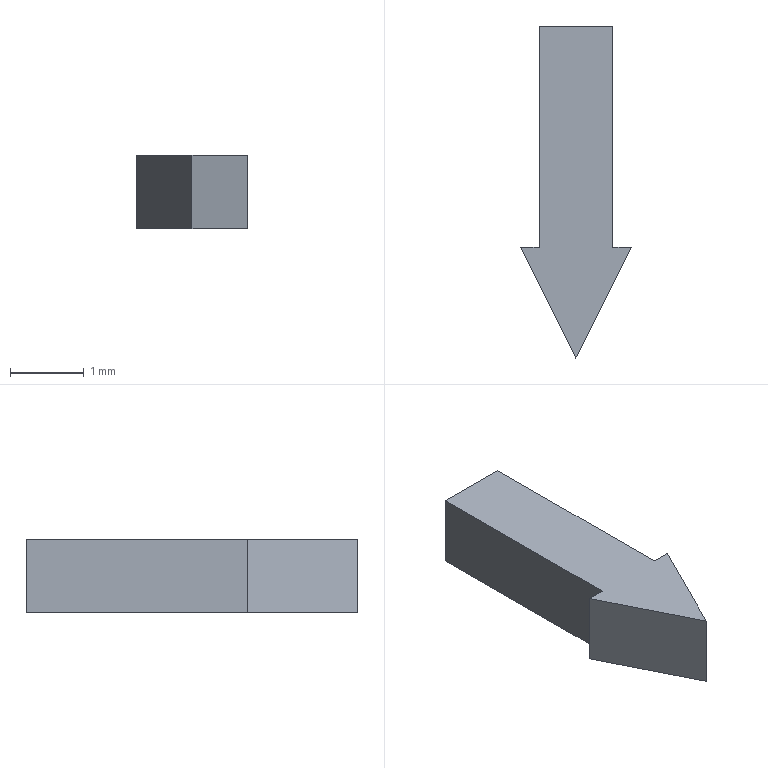Part | STEP file | OP-85138-Part-2-3 | 1 solid | 9 faces | box 1.5 x 4.5 x 1 mm | volume 4.125 mm3 | plane 9
STEP:
#1=CARTESIAN_POINT('',(3.75,2.25,0.));
#2=VERTEX_POINT('',#1);
#3=CARTESIAN_POINT('',(3.5,2.25,0.));
#4=VERTEX_POINT('',#3);
#5=CARTESIAN_POINT('',(3.,2.25,0.));
#6=DIRECTION('',(-1.,0.,0.));
#7=VECTOR('',#6,1000.);
#8=LINE('',#5,#7);
#9=EDGE_CURVE('',#2,#4,#8,.T.);
#10=ORIENTED_EDGE('',*,*,#9,.T.);
#11=CARTESIAN_POINT('',(3.5,2.25,1.));
#12=VERTEX_POINT('',#11);
#13=CARTESIAN_POINT('',(3.5,2.25,0.));
#14=DIRECTION('',(0.,0.,1.));
#15=VECTOR('',#14,1000.);
#16=LINE('',#13,#15);
#17=EDGE_CURVE('',#4,#12,#16,.T.);
#18=ORIENTED_EDGE('',*,*,#17,.T.);
#19=CARTESIAN_POINT('',(3.75,2.25,1.));
#20=VERTEX_POINT('',#19);
#21=CARTESIAN_POINT('',(3.,2.25,1.));
#22=DIRECTION('',(1.,0.,0.));
#23=VECTOR('',#22,1000.);
#24=LINE('',#21,#23);
#25=EDGE_CURVE('',#12,#20,#24,.T.);
#26=ORIENTED_EDGE('',*,*,#25,.T.);
#27=CARTESIAN_POINT('',(3.75,2.25,0.));
#28=DIRECTION('',(0.,0.,1.));
#29=VECTOR('',#28,1000.);
#30=LINE('',#27,#29);
#31=EDGE_CURVE('',#2,#20,#30,.T.);
#32=ORIENTED_EDGE('',*,*,#31,.F.);
#33=EDGE_LOOP('',(#10,#18,#26,#32));
#34=FACE_OUTER_BOUND('',#33,.T.);
#35=CARTESIAN_POINT('',(3.,2.25,0.));
#36=DIRECTION('',(0.,1.,0.));
#37=DIRECTION('',(0.,0.,-1.));
#38=AXIS2_PLACEMENT_3D('',#35,#36,#37);
#39=PLANE('',#38);
#40=ADVANCED_FACE('',(#34),#39,.T.);
#41=CARTESIAN_POINT('',(2.25,2.25,1.));
#42=VERTEX_POINT('',#41);
#43=CARTESIAN_POINT('',(2.5,2.25,1.));
#44=VERTEX_POINT('',#43);
#45=CARTESIAN_POINT('',(3.,2.25,1.));
#46=DIRECTION('',(1.,0.,0.));
#47=VECTOR('',#46,1000.);
#48=LINE('',#45,#47);
#49=EDGE_CURVE('',#42,#44,#48,.T.);
#50=ORIENTED_EDGE('',*,*,#49,.F.);
#51=CARTESIAN_POINT('',(3.,0.75,1.));
#52=VERTEX_POINT('',#51);
#53=CARTESIAN_POINT('',(2.7,1.35,1.));
#54=DIRECTION('',(0.4472,-0.8944,0.));
#55=VECTOR('',#54,1000.);
#56=LINE('',#53,#55);
#57=EDGE_CURVE('',#42,#52,#56,.T.);
#58=ORIENTED_EDGE('',*,*,#57,.T.);
#59=CARTESIAN_POINT('',(3.3,1.35,1.));
#60=DIRECTION('',(0.4472,0.8944,0.));
#61=VECTOR('',#60,1000.);
#62=LINE('',#59,#61);
#63=EDGE_CURVE('',#52,#20,#62,.T.);
#64=ORIENTED_EDGE('',*,*,#63,.T.);
#65=ORIENTED_EDGE('',*,*,#25,.F.);
#66=CARTESIAN_POINT('',(3.5,5.25,1.));
#67=VERTEX_POINT('',#66);
#68=CARTESIAN_POINT('',(3.5,3.75,1.));
#69=DIRECTION('',(0.,-1.,0.));
#70=VECTOR('',#69,1000.);
#71=LINE('',#68,#70);
#72=EDGE_CURVE('',#67,#12,#71,.T.);
#73=ORIENTED_EDGE('',*,*,#72,.F.);
#74=CARTESIAN_POINT('',(2.5,5.25,1.));
#75=VERTEX_POINT('',#74);
#76=CARTESIAN_POINT('',(3.,5.25,1.));
#77=DIRECTION('',(1.,0.,0.));
#78=VECTOR('',#77,1000.);
#79=LINE('',#76,#78);
#80=EDGE_CURVE('',#75,#67,#79,.T.);
#81=ORIENTED_EDGE('',*,*,#80,.F.);
#82=CARTESIAN_POINT('',(2.5,3.75,1.));
#83=DIRECTION('',(0.,1.,0.));
#84=VECTOR('',#83,1000.);
#85=LINE('',#82,#84);
#86=EDGE_CURVE('',#44,#75,#85,.T.);
#87=ORIENTED_EDGE('',*,*,#86,.F.);
#88=EDGE_LOOP('',(#50,#58,#64,#65,#73,#81,#87));
#89=FACE_OUTER_BOUND('',#88,.T.);
#90=CARTESIAN_POINT('',(3.,1.5,1.));
#91=DIRECTION('',(0.,0.,1.));
#92=DIRECTION('',(0.,1.,0.));
#93=AXIS2_PLACEMENT_3D('',#90,#91,#92);
#94=PLANE('',#93);
#95=ADVANCED_FACE('',(#89),#94,.T.);
#96=CARTESIAN_POINT('',(3.,0.75,0.));
#97=VERTEX_POINT('',#96);
#98=CARTESIAN_POINT('',(3.3,1.35,0.));
#99=DIRECTION('',(-0.4472,-0.8944,0.));
#100=VECTOR('',#99,1000.);
#101=LINE('',#98,#100);
#102=EDGE_CURVE('',#2,#97,#101,.T.);
#103=ORIENTED_EDGE('',*,*,#102,.T.);
#104=CARTESIAN_POINT('',(2.25,2.25,0.));
#105=VERTEX_POINT('',#104);
#106=CARTESIAN_POINT('',(2.7,1.35,0.));
#107=DIRECTION('',(-0.4472,0.8944,0.));
#108=VECTOR('',#107,1000.);
#109=LINE('',#106,#108);
#110=EDGE_CURVE('',#97,#105,#109,.T.);
#111=ORIENTED_EDGE('',*,*,#110,.T.);
#112=CARTESIAN_POINT('',(2.5,2.25,0.));
#113=VERTEX_POINT('',#112);
#114=CARTESIAN_POINT('',(3.,2.25,0.));
#115=DIRECTION('',(-1.,0.,0.));
#116=VECTOR('',#115,1000.);
#117=LINE('',#114,#116);
#118=EDGE_CURVE('',#113,#105,#117,.T.);
#119=ORIENTED_EDGE('',*,*,#118,.F.);
#120=CARTESIAN_POINT('',(2.5,5.25,0.));
#121=VERTEX_POINT('',#120);
#122=CARTESIAN_POINT('',(2.5,3.75,0.));
#123=DIRECTION('',(0.,-1.,0.));
#124=VECTOR('',#123,1000.);
#125=LINE('',#122,#124);
#126=EDGE_CURVE('',#121,#113,#125,.T.);
#127=ORIENTED_EDGE('',*,*,#126,.F.);
#128=CARTESIAN_POINT('',(3.5,5.25,0.));
#129=VERTEX_POINT('',#128);
#130=CARTESIAN_POINT('',(3.,5.25,0.));
#131=DIRECTION('',(-1.,0.,0.));
#132=VECTOR('',#131,1000.);
#133=LINE('',#130,#132);
#134=EDGE_CURVE('',#129,#121,#133,.T.);
#135=ORIENTED_EDGE('',*,*,#134,.F.);
#136=CARTESIAN_POINT('',(3.5,3.75,0.));
#137=DIRECTION('',(0.,1.,0.));
#138=VECTOR('',#137,1000.);
#139=LINE('',#136,#138);
#140=EDGE_CURVE('',#4,#129,#139,.T.);
#141=ORIENTED_EDGE('',*,*,#140,.F.);
#142=ORIENTED_EDGE('',*,*,#9,.F.);
#143=EDGE_LOOP('',(#103,#111,#119,#127,#135,#141,#142));
#144=FACE_OUTER_BOUND('',#143,.T.);
#145=CARTESIAN_POINT('',(3.,1.5,0.));
#146=DIRECTION('',(0.,0.,-1.));
#147=DIRECTION('',(0.,-1.,0.));
#148=AXIS2_PLACEMENT_3D('',#145,#146,#147);
#149=PLANE('',#148);
#150=ADVANCED_FACE('',(#144),#149,.T.);
#151=CARTESIAN_POINT('',(2.5,2.25,0.));
#152=DIRECTION('',(0.,0.,1.));
#153=VECTOR('',#152,1000.);
#154=LINE('',#151,#153);
#155=EDGE_CURVE('',#113,#44,#154,.T.);
#156=ORIENTED_EDGE('',*,*,#155,.F.);
#157=ORIENTED_EDGE('',*,*,#118,.T.);
#158=CARTESIAN_POINT('',(2.25,2.25,0.));
#159=DIRECTION('',(0.,0.,1.));
#160=VECTOR('',#159,1000.);
#161=LINE('',#158,#160);
#162=EDGE_CURVE('',#105,#42,#161,.T.);
#163=ORIENTED_EDGE('',*,*,#162,.T.);
#164=ORIENTED_EDGE('',*,*,#49,.T.);
#165=EDGE_LOOP('',(#156,#157,#163,#164));
#166=FACE_OUTER_BOUND('',#165,.T.);
#167=CARTESIAN_POINT('',(3.,2.25,0.));
#168=DIRECTION('',(0.,1.,0.));
#169=DIRECTION('',(0.,0.,-1.));
#170=AXIS2_PLACEMENT_3D('',#167,#168,#169);
#171=PLANE('',#170);
#172=ADVANCED_FACE('',(#166),#171,.T.);
#173=ORIENTED_EDGE('',*,*,#102,.F.);
#174=ORIENTED_EDGE('',*,*,#31,.T.);
#175=ORIENTED_EDGE('',*,*,#63,.F.);
#176=CARTESIAN_POINT('',(3.,0.75,0.));
#177=DIRECTION('',(0.,0.,1.));
#178=VECTOR('',#177,1000.);
#179=LINE('',#176,#178);
#180=EDGE_CURVE('',#97,#52,#179,.T.);
#181=ORIENTED_EDGE('',*,*,#180,.F.);
#182=EDGE_LOOP('',(#173,#174,#175,#181));
#183=FACE_OUTER_BOUND('',#182,.T.);
#184=CARTESIAN_POINT('',(3.,0.75,0.));
#185=DIRECTION('',(-0.8944,0.4472,0.));
#186=DIRECTION('',(0.,0.,1.));
#187=AXIS2_PLACEMENT_3D('',#184,#185,#186);
#188=PLANE('',#187);
#189=ADVANCED_FACE('',(#183),#188,.F.);
#190=ORIENTED_EDGE('',*,*,#110,.F.);
#191=ORIENTED_EDGE('',*,*,#180,.T.);
#192=ORIENTED_EDGE('',*,*,#57,.F.);
#193=ORIENTED_EDGE('',*,*,#162,.F.);
#194=EDGE_LOOP('',(#190,#191,#192,#193));
#195=FACE_OUTER_BOUND('',#194,.T.);
#196=CARTESIAN_POINT('',(2.25,2.25,0.));
#197=DIRECTION('',(0.8944,0.4472,0.));
#198=DIRECTION('',(0.,0.,1.));
#199=AXIS2_PLACEMENT_3D('',#196,#197,#198);
#200=PLANE('',#199);
#201=ADVANCED_FACE('',(#195),#200,.F.);
#202=CARTESIAN_POINT('',(3.5,5.25,0.));
#203=DIRECTION('',(0.,0.,1.));
#204=VECTOR('',#203,1000.);
#205=LINE('',#202,#204);
#206=EDGE_CURVE('',#129,#67,#205,.T.);
#207=ORIENTED_EDGE('',*,*,#206,.T.);
#208=ORIENTED_EDGE('',*,*,#72,.T.);
#209=ORIENTED_EDGE('',*,*,#17,.F.);
#210=ORIENTED_EDGE('',*,*,#140,.T.);
#211=EDGE_LOOP('',(#207,#208,#209,#210));
#212=FACE_OUTER_BOUND('',#211,.T.);
#213=CARTESIAN_POINT('',(3.5,3.75,0.));
#214=DIRECTION('',(1.,0.,0.));
#215=DIRECTION('',(0.,0.,-1.));
#216=AXIS2_PLACEMENT_3D('',#213,#214,#215);
#217=PLANE('',#216);
#218=ADVANCED_FACE('',(#212),#217,.T.);
#219=ORIENTED_EDGE('',*,*,#155,.T.);
#220=ORIENTED_EDGE('',*,*,#86,.T.);
#221=CARTESIAN_POINT('',(2.5,5.25,0.));
#222=DIRECTION('',(0.,0.,1.));
#223=VECTOR('',#222,1000.);
#224=LINE('',#221,#223);
#225=EDGE_CURVE('',#121,#75,#224,.T.);
#226=ORIENTED_EDGE('',*,*,#225,.F.);
#227=ORIENTED_EDGE('',*,*,#126,.T.);
#228=EDGE_LOOP('',(#219,#220,#226,#227));
#229=FACE_OUTER_BOUND('',#228,.T.);
#230=CARTESIAN_POINT('',(2.5,3.75,0.));
#231=DIRECTION('',(-1.,0.,0.));
#232=DIRECTION('',(0.,0.,1.));
#233=AXIS2_PLACEMENT_3D('',#230,#231,#232);
#234=PLANE('',#233);
#235=ADVANCED_FACE('',(#229),#234,.T.);
#236=ORIENTED_EDGE('',*,*,#134,.T.);
#237=ORIENTED_EDGE('',*,*,#225,.T.);
#238=ORIENTED_EDGE('',*,*,#80,.T.);
#239=ORIENTED_EDGE('',*,*,#206,.F.);
#240=EDGE_LOOP('',(#236,#237,#238,#239));
#241=FACE_OUTER_BOUND('',#240,.T.);
#242=CARTESIAN_POINT('',(3.,5.25,0.));
#243=DIRECTION('',(0.,1.,0.));
#244=DIRECTION('',(0.,0.,-1.));
#245=AXIS2_PLACEMENT_3D('',#242,#243,#244);
#246=PLANE('',#245);
#247=ADVANCED_FACE('',(#241),#246,.T.);
#248=CLOSED_SHELL('',(#40,#95,#150,#172,#189,#201,#218,#235,#247));
#249=MANIFOLD_SOLID_BREP('',#248);
#250=CARTESIAN_POINT('',(0.,0.,0.));
#251=DIRECTION('',(0.,0.,1.));
#252=DIRECTION('',(1.,0.,0.));
#253=AXIS2_PLACEMENT_3D('',#250,#251,#252);
#254=(LENGTH_UNIT()NAMED_UNIT(*)SI_UNIT(.MILLI.,.METRE.));
#255=UNCERTAINTY_MEASURE_WITH_UNIT(LENGTH_MEASURE(0.00001),#254,'','');
#256=(NAMED_UNIT(*)PLANE_ANGLE_UNIT()SI_UNIT($,.RADIAN.));
#257=(NAMED_UNIT(*)SI_UNIT($,.STERADIAN.)SOLID_ANGLE_UNIT());
#258=(GEOMETRIC_REPRESENTATION_CONTEXT(3)GLOBAL_UNCERTAINTY_ASSIGNED_CONTEXT((#255))GLOBAL_UNIT_ASSIGNED_CONTEXT((#254,#256,#257))REPRESENTATION_CONTEXT('',''));
#259=ADVANCED_BREP_SHAPE_REPRESENTATION('',(#249,#253),#258);